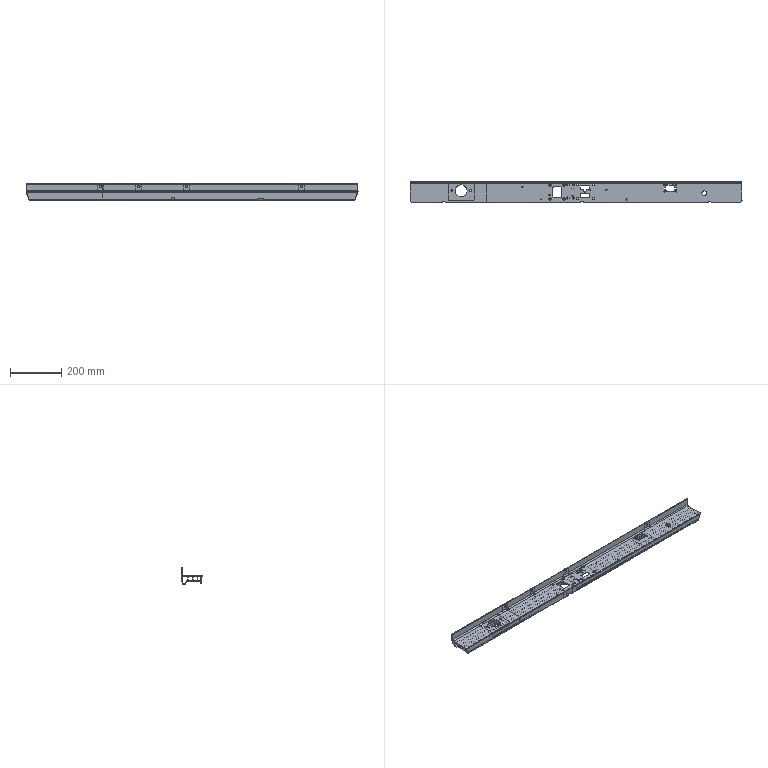NC program | NX | posted with a generic post | part box 1301 x 81.1 x 63 mm
Lines 4351 to 5403 of 19512:
(FLOOR_WALL , TOOL : D10)
N8682 T10 M6
N8684 G54
N8686 G17 G0 G90 X655.75 Y37.25 B0. C0. S6000 M3
N8688 G43 Z30. H10
N8690 Z-28.5
N8692 G94 G1 Z-30. F1000.
N8694 X653.384 Y36.253
N8696 G3 X654.25 Y35.753 R1.
N8698 G1 X450.
N8700 Y36.368
N8702 X654.25
N8704 Y36.983
N8706 X450.
N8708 Y37.597
N8710 X654.25
N8712 Y38.212
N8714 X450.
N8716 Y38.827
N8718 X654.25
N8720 Y39.442
N8722 X450.
N8724 Y40.057
N8726 X654.25
N8728 G2 X655.116 Y39.557 R1.
N8730 G1 X655.75 Y38.458
N8732 Z-28.5
N8734 G0 Z30.
N8736 X17.795 Y40.349
N8738 Z-25.5
N8740 G1 X1.001 Z-30.
N8742 X406.
N8744 Y35.75
N8746 X1.001
N8748 Z-28.5
N8750 G0 Z30.
N8752 X-169.205 Y40.349
N8754 Z-25.5
N8756 G1 X-185.999 Z-30.
N8758 X-42.999
N8760 Y35.75
N8762 X-185.999
N8764 Z-28.5
N8766 G0 Z30.
N8768 X-319.205 Y40.337
N8770 Z-25.5
N8772 G1 X-335.999 Z-30.
N8774 X-229.999
N8776 Y35.75
N8778 X-335.999
N8780 Z-28.5
N8782 G0 Z30.
N8784 X-655.748 Y41.916
N8786 Z-28.5
N8788 G1 Z-30.
N8790 X-655.114 Y40.817
N8792 G3 X-654.248 Y40.317 R1.
N8794 G1 X-379.999
N8796 Y35.75
N8798 X-654.248
N8800 G2 X-655.114 Y36.25 R1.
N8802 G1 X-655.748 Y37.348
N8804 Z-28.5
N8806 G0 Z30.
(11 , TOOL : D10)
N8808 X409.174 Y30.201 S5500
N8810 Z-9.5
N8812 G1 Z-12.5 F500.
N8814 X410.501 Y30.968
N8816 G3 X411.001 Y31.834 R1.
N8818 G1 X411. Y37.634 F1000.
N8820 Y40.25
N8822 X411.001 Y45.22
N8824 X411.002 Y45.666
N8826 G3 X410.504 Y46.534 R1.
N8828 G1 X409.176 Y47.304
N8830 Z-9.5
N8832 G0 X409.172 Y30.202 Z-22.
N8834 G1 Z-25. F500.
N8836 X410.499 Y30.968
N8838 G3 X410.999 Y31.834 R1.
N8840 G1 X411. Y37.634 F1000.
N8842 Y40.25
N8844 X410.997 Y40.577
N8846 Y44.774
N8848 X411.001 Y45.666
N8850 G3 X410.505 Y46.535 R1.
N8852 G1 X409.177 Y47.31
N8854 Z-22.
N8856 G0 Z30.
N8858 X446.825 Y47.299
N8860 Z-9.5
N8862 G1 Z-12.5 F500.
N8864 X445.498 Y46.533
N8866 G3 X444.998 Y45.666 R1.
N8868 G1 X445. Y40.25 F1000.
N8870 Y37.634
N8872 X444.998 Y31.834
N8874 G3 X445.498 Y30.968 R1.
N8876 G1 X446.826 Y30.201
N8878 Z-9.5
N8880 G0 Y47.299 Z-22.
N8882 G1 Z-25. F500.
N8884 X445.499 Y46.533
N8886 G3 X444.999 Y45.666 R1.
N8888 G1 X445. Y41.65 F1000.
N8890 X445.003 Y40.758
N8892 X444.981 Y40.687
N8894 X445.003 Y40.674
N8896 X445. Y40.25
N8898 Y37.634
N8900 X445.004 Y37.188
N8902 X445. Y31.834
N8904 G3 X445.499 Y30.967 R1.
N8906 G1 X446.827 Y30.2
N8908 Z-22.
N8910 G0 Z30.
N8912 X-39.825 Y30.201
N8914 Z-9.5
N8916 G1 Z-12.5 F500.
N8918 X-38.498 Y30.968
N8920 G3 X-37.998 Y31.834 R1.
N8922 G1 X-37.999 Y37.634 F1000.
N8924 Y40.25
N8926 X-37.998 Y45.22
N8928 X-37.997 Y45.666
N8930 G3 X-38.495 Y46.534 R1.
N8932 G1 X-39.823 Y47.304
N8934 Z-9.5
N8936 G0 X-39.827 Y30.202 Z-22.
N8938 G1 Z-25. F500.
N8940 X-38.5 Y30.968
N8942 G3 X-38. Y31.834 R1.
N8944 G1 X-37.999 Y37.634 F1000.
N8946 Y40.25
N8948 X-38.003 Y40.577
N8950 X-38.002 Y44.774
N8952 X-37.998 Y45.666
N8954 G3 X-38.494 Y46.535 R1.
N8956 G1 X-39.822 Y47.31
N8958 Z-22.
N8960 G0 Z30.
N8962 X-2.174 Y47.299
N8964 Z-9.5
N8966 G1 Z-12.5 F500.
N8968 X-3.501 Y46.533
N8970 G3 X-4.001 Y45.666 R1.
N8972 G1 X-3.999 Y40.25 F1000.
N8974 Y37.634
N8976 X-4.001 Y31.778
N8978 G3 X-3.501 Y30.912 R1.
N8980 G1 X-2.185 Y30.152
N8982 Z-9.5
N8984 G0 X-2.173 Y47.299 Z-22.
N8986 G1 Z-25. F500.
N8988 X-3.5 Y46.533
N8990 G3 X-4. Y45.666 R1.
N8992 G1 X-3.999 Y41.65 F1000.
N8994 X-3.996 Y40.758
N8996 X-4.019 Y40.687
N8998 X-3.996 Y40.674
N9000 X-3.999 Y40.25
N9002 Y37.634
N9004 X-3.996 Y37.188
N9006 X-3.999 Y31.778
N9008 G3 X-3.5 Y30.911 R1.
N9010 G1 X-2.184 Y30.151
N9012 Z-22.
N9014 G0 Z30.
N9016 X-226.825 Y30.201
N9018 Z-9.5
N9020 G1 Z-12.5 F500.
N9022 X-225.498 Y30.968
N9024 G3 X-224.998 Y31.834 R1.
N9026 G1 X-224.999 Y37.634 F1000.
N9028 Y40.25
N9030 X-224.998 Y45.22
N9032 X-224.997 Y45.666
N9034 G3 X-225.495 Y46.534 R1.
N9036 G1 X-226.823 Y47.304
N9038 Z-9.5
N9040 G0 X-226.827 Y30.2 Z-22.
N9042 G1 Z-25. F500.
N9044 X-225.499 Y30.967
N9046 G3 X-225. Y31.834 R1.
N9048 G1 X-225.003 Y37.188 F1000.
N9050 X-224.999 Y37.634
N9052 Y40.25
N9054 X-225.003 Y40.577
N9056 X-225.002 Y44.774
N9058 X-224.998 Y45.666
N9060 G3 X-225.494 Y46.535 R1.
N9062 G1 X-226.822 Y47.31
N9064 Z-22.
N9066 G0 Z30.
N9068 X-189.174 Y47.299
N9070 Z-9.5
N9072 G1 Z-12.5 F500.
N9074 X-190.501 Y46.533
N9076 G3 X-191.001 Y45.666 R1.
N9078 G1 X-190.999 Y40.25 F1000.
N9080 Y37.634
N9082 X-191.001 Y31.834
N9084 G3 X-190.501 Y30.968 R1.
N9086 G1 X-189.174 Y30.201
N9088 Z-9.5
N9090 G0 X-189.173 Y47.299 Z-22.
N9092 G1 Z-25. F500.
N9094 X-190.5 Y46.533
N9096 G3 X-191. Y45.666 R1.
N9098 G1 X-190.999 Y41.65 F1000.
N9100 X-190.996 Y40.758
N9102 X-191.019 Y40.687
N9104 X-190.996 Y40.674
N9106 X-190.999 Y40.25
N9108 Y37.634
N9110 X-190.996 Y37.188
N9112 X-190.999 Y31.834
N9114 G3 X-190.5 Y30.967 R1.
N9116 G1 X-189.172 Y30.2
N9118 Z-22.
N9120 G0 Z30.
N9122 X-376.825 Y30.201
N9124 Z-9.5
N9126 G1 Z-12.5 F500.
N9128 X-375.498 Y30.968
N9130 G3 X-374.998 Y31.834 R1.
N9132 G1 X-374.999 Y37.634 F1000.
N9134 Y40.25
N9136 X-374.998 Y45.22
N9138 X-374.997 Y45.666
N9140 G3 X-375.495 Y46.534 R1.
N9142 G1 X-376.823 Y47.304
N9144 Z-9.5
N9146 G0 X-376.827 Y30.2 Z-22.
N9148 G1 Z-25. F500.
N9150 X-375.499 Y30.967
N9152 G3 X-375. Y31.834 R1.
N9154 G1 X-375.003 Y37.188 F1000.
N9156 X-374.999 Y37.634
N9158 Y40.25
N9160 X-375.003 Y40.577
N9162 X-375.002 Y44.774
N9164 X-374.998 Y45.666
N9166 G3 X-375.494 Y46.535 R1.
N9168 G1 X-376.822 Y47.31
N9170 Z-22.
N9172 G0 Z30.
N9174 X-339.174 Y47.299
N9176 Z-9.5
N9178 G1 Z-12.5 F500.
N9180 X-340.501 Y46.533
N9182 G3 X-341.001 Y45.666 R1.
N9184 G1 X-340.999 Y40.25 F1000.
N9186 Y37.634
N9188 X-341.001 Y31.834
N9190 G3 X-340.501 Y30.968 R1.
N9192 G1 X-339.174 Y30.201
N9194 Z-9.5
N9196 G0 X-339.173 Y47.3 Z-22.
N9198 G1 Z-25. F500.
N9200 X-340.501 Y46.533
N9202 G3 X-341. Y45.666 R1.
N9204 G1 X-340.996 Y40.758 F1000.
N9206 X-341.019 Y40.687
N9208 X-340.996 Y40.674
N9210 X-340.999 Y40.25
N9212 Y37.634
N9214 X-340.996 Y37.188
N9216 X-340.999 Y31.834
N9218 G3 X-340.5 Y30.967 R1.
N9220 G1 X-339.172 Y30.2
N9222 Z-22.
N9224 G0 Z30.
(FLOOR_WALL_COPY , TOOL : D10)
N9226 X-494.633 Y32.747 S6000
N9228 Z-28.8
N9230 G1 Z-30.3
N9232 G3 X-495.5 Y33.247 R1.
N9234 G1 X-404.5
N9236 Y28.532
N9238 X-495.5
N9240 Y23.817
N9242 X-404.5
N9244 Y19.102
N9246 X-495.5
N9248 Y14.386
N9250 X-404.5
N9252 Y9.671
N9254 X-495.5
N9256 Y4.956
N9258 X-404.5
N9260 Y0.241
N9262 X-495.5
N9264 Y-4.474
N9266 X-404.5
N9268 Y-9.189
N9270 X-495.5
N9272 Y-13.905
N9274 X-404.5
N9276 Y-18.62
N9278 X-495.5
N9280 Y-23.335
N9282 X-404.5
N9284 Y-28.05
N9286 X-495.5
N9288 Y-27.184
N9290 G3 X-496. Y-28.05 R1.
N9292 G1 Y-28.55
N9294 X-404.
N9296 Y33.75
N9298 X-496.
N9300 Y-28.05
N9302 G3 X-495.75 Y-28.483 R0.5
N9304 G1 X-494.5 Y-27.05
N9306 Z-28.8
N9308 G0 Z30.
(ZLEVEL_PROFILE_COPY_2 , TOOL : D10)
N9310 X-63.3 Y5.083
N9312 Z-28.5
N9314 G1 Y15.285 Z-29.035
N9316 X-63.353 Y15.284 Z-29.038
N9318 X-85.347 Z-30.19
N9320 X-85.4 Y15.285 Z-30.193
N9322 Y-0.115 Z-31.
N9324 Y-15.516 F2000.
N9326 X-63.3
N9328 Y15.285
N9330 X-63.353 Y15.284
N9332 X-85.347
N9334 X-85.4 Y15.285
N9336 Y-0.115
N9338 Y-15.516 Z-31.269
N9340 X-63.3 Z-31.655
N9342 Y4.273 Z-32.
N9344 Y15.285
N9346 X-63.353 Y15.284
N9348 X-85.347
N9350 X-85.4 Y15.285
N9352 Y-0.115
N9354 Y-15.516 Z-32.269
N9356 X-63.3 Z-32.655
N9358 Y4.273 Z-33.
N9360 Y15.285
N9362 X-63.353 Y15.284
N9364 X-85.347
N9366 X-85.4 Y15.285
N9368 Y-15.516
N9370 X-63.3
N9372 Y4.273
N9374 Z-31.5
N9376 G0 Z30.
N9378 X47.5 Y-15.102
N9380 Z-28.5
N9382 G1 Y-10.702 Z-28.731 F1000.
N9384 X47.456 Y-10.704 Z-28.733
N9386 X22.543 Z-30.039
N9388 X22.5 Y-10.702 Z-30.041
N9390 Y-16.504 Z-30.345
N9392 X35. Z-31.
N9394 X47.5 F2000.
N9396 Y-10.702
N9398 X47.456 Y-10.704
N9400 X22.543
N9402 X22.5 Y-10.702
N9404 Y-16.504
N9406 X35.
N9408 X47.5 Z-31.271
N9410 Y-10.789 Z-31.394
N9412 Y-10.704 Z-31.396
N9414 X47.143 Z-31.404
N9416 X22.708 Z-31.933
N9418 X22.5 Z-31.937
N9420 Y-10.938 Z-31.942
N9422 Y-13.603 Z-32.
N9424 Y-16.504
N9426 X35.
N9428 X47.5 Z-32.271
N9430 Y-10.789 Z-32.394
N9432 Y-10.704 Z-32.396
N9434 X47.143 Z-32.404
N9436 X22.708 Z-32.933
N9438 X22.5 Z-32.937
N9440 Y-10.938 Z-32.942
N9442 Y-13.603 Z-33.
N9444 Y-16.504
N9446 X47.5
N9448 Y-10.702
N9450 X47.456 Y-10.704
N9452 X22.543
N9454 X22.5 Y-10.702
N9456 Y-13.603
N9458 Z-31.5
N9460 G0 Z30.
N9462 X22.827 Y14.996
N9464 Z-28.5
N9466 G1 X29.896 Z-28.871 F1000.
N9468 X30.779 Y14.87 Z-28.917
N9470 X31.631 Y14.603 Z-28.964
N9472 X32.428 Y14.203 Z-29.011
N9474 X33.15 Y13.679 Z-29.058
N9476 X33.778 Y13.046 Z-29.104
N9478 X34.296 Y12.319 Z-29.151
N9480 X34.689 Y11.519 Z-29.198
N9482 X34.949 Y10.665 Z-29.245
N9484 X35. Y10.338 Z-29.262
N9486 X35.05 Y10.665 Z-29.279
N9488 X35.31 Y11.519 Z-29.326
N9490 X35.703 Y12.319 Z-29.373
N9492 X36.221 Y13.046 Z-29.42
N9494 X36.849 Y13.679 Z-29.466
N9496 X37.571 Y14.203 Z-29.513
N9498 X38.369 Y14.603 Z-29.56
N9500 X39.22 Y14.87 Z-29.607
N9502 X40.103 Y14.996 Z-29.653
N9504 X47.5 Z-30.041
N9506 Y20.796 Z-30.345
N9508 X35. Z-31.
N9510 X22.5 F2000.
N9512 Y14.996
N9514 X29.564
N9516 G2 X35. Y10.338 R5.5
N9518 X40.435 Y14.996 R5.5
N9520 G1 X47.5
N9522 Y20.796
N9524 X35.
N9526 X22.509 Z-31.251
N9528 X22.5 Y20.582 Z-31.256
N9530 Y15.006 Z-31.368
N9532 X22.712 Y14.996 Z-31.372
N9534 X29.403 Z-31.507
N9536 X29.626 Y14.995 Z-31.511
N9538 X29.849 Y14.988 Z-31.516
N9540 X30.072 Y14.972 Z-31.52
N9542 X30.293 Y14.947 Z-31.525
N9544 X30.514 Y14.913 Z-31.529
N9546 X30.733 Y14.87 Z-31.534
N9548 X30.95 Y14.818 Z-31.538
N9550 X31.164 Y14.758 Z-31.543
N9552 X31.376 Y14.689 Z-31.547
N9554 X31.585 Y14.611 Z-31.552
N9556 X31.791 Y14.525 Z-31.556
N9558 X31.993 Y14.43 Z-31.561
N9560 X32.191 Y14.328 Z-31.565
N9562 X32.385 Y14.217 Z-31.57
N9564 X32.574 Y14.099 Z-31.574
N9566 X32.758 Y13.973 Z-31.579
N9568 X32.937 Y13.84 Z-31.583
N9570 X33.11 Y13.7 Z-31.588
N9572 X33.278 Y13.553 Z-31.592
N9574 X33.439 Y13.399 Z-31.597
N9576 X33.594 Y13.238 Z-31.601
N9578 X33.743 Y13.072 Z-31.606
N9580 X33.884 Y12.9 Z-31.61
N9582 X34.019 Y12.722 Z-31.615
N9584 X34.146 Y12.538 Z-31.619
N9586 X34.266 Y12.35 Z-31.623
N9588 X34.378 Y12.157 Z-31.628
N9590 X34.481 Y11.96 Z-31.632
N9592 X34.577 Y11.759 Z-31.637
N9594 X34.665 Y11.553 Z-31.641
N9596 X34.744 Y11.345 Z-31.646
N9598 X34.815 Y11.133 Z-31.65
N9600 X34.877 Y10.919 Z-31.655
N9602 X34.93 Y10.703 Z-31.659
N9604 X34.975 Y10.484 Z-31.664
N9606 X35.012 Y10.411 Z-31.668
N9608 X35.053 Y10.63 Z-31.673
N9610 X35.103 Y10.847 Z-31.677
N9612 X35.163 Y11.062 Z-31.682
N9614 X35.231 Y11.275 Z-31.686
N9616 X35.307 Y11.484 Z-31.691
N9618 X35.392 Y11.691 Z-31.695
N9620 X35.485 Y11.893 Z-31.7
N9622 X35.586 Y12.092 Z-31.704
N9624 X35.695 Y12.286 Z-31.709
N9626 X35.812 Y12.476 Z-31.713
N9628 X35.937 Y12.661 Z-31.718
N9630 X36.069 Y12.841 Z-31.722
N9632 X36.208 Y13.015 Z-31.727
N9634 X36.355 Y13.184 Z-31.731
N9636 X36.507 Y13.346 Z-31.736
N9638 X36.667 Y13.502 Z-31.74
N9640 X36.832 Y13.652 Z-31.745
N9642 X37.004 Y13.794 Z-31.749
N9644 X37.181 Y13.93 Z-31.754
N9646 X37.363 Y14.058 Z-31.758
N9648 X37.551 Y14.179 Z-31.762
N9650 X37.743 Y14.292 Z-31.767
N9652 X37.94 Y14.397 Z-31.771
N9654 X38.14 Y14.494 Z-31.776
N9656 X38.345 Y14.583 Z-31.78
N9658 X38.553 Y14.664 Z-31.785
N9660 X38.764 Y14.736 Z-31.789
N9662 X38.978 Y14.799 Z-31.794
N9664 X39.194 Y14.854 Z-31.798
N9666 X39.412 Y14.9 Z-31.803
N9668 X39.632 Y14.937 Z-31.807
N9670 X39.853 Y14.965 Z-31.812
N9672 X40.076 Y14.984 Z-31.816
N9674 X40.298 Y14.994 Z-31.821
N9676 X40.522 Y14.996 Z-31.825
N9678 X47.436 Z-31.964
N9680 X47.5 Y15.155 Z-31.969
N9682 Y16.716 Z-32.
N9684 Y20.796
N9686 X35.
N9688 X22.509 Z-32.251
N9690 X22.5 Y20.582 Z-32.256
N9692 Y15.006 Z-32.368
N9694 X22.712 Y14.996 Z-32.372
N9696 X29.403 Z-32.507
N9698 X29.626 Y14.995 Z-32.511
N9700 X29.849 Y14.988 Z-32.516
N9702 X30.072 Y14.972 Z-32.52
N9704 X30.293 Y14.947 Z-32.525
N9706 X30.514 Y14.913 Z-32.529
N9708 X30.733 Y14.87 Z-32.534
N9710 X30.95 Y14.818 Z-32.538
N9712 X31.164 Y14.758 Z-32.543
N9714 X31.376 Y14.689 Z-32.547
N9716 X31.585 Y14.611 Z-32.552
N9718 X31.791 Y14.525 Z-32.556
N9720 X31.993 Y14.43 Z-32.561
N9722 X32.191 Y14.328 Z-32.565
N9724 X32.385 Y14.217 Z-32.57
N9726 X32.574 Y14.099 Z-32.574
N9728 X32.758 Y13.973 Z-32.579
N9730 X32.937 Y13.84 Z-32.583
N9732 X33.11 Y13.7 Z-32.588
N9734 X33.278 Y13.553 Z-32.592
N9736 X33.439 Y13.399 Z-32.597
N9738 X33.594 Y13.238 Z-32.601
N9740 X33.743 Y13.072 Z-32.606
N9742 X33.884 Y12.9 Z-32.61
N9744 X34.019 Y12.722 Z-32.615
N9746 X34.146 Y12.538 Z-32.619
N9748 X34.266 Y12.35 Z-32.623
N9750 X34.378 Y12.157 Z-32.628
N9752 X34.481 Y11.96 Z-32.632
N9754 X34.577 Y11.759 Z-32.637
N9756 X34.665 Y11.553 Z-32.641
N9758 X34.744 Y11.345 Z-32.646
N9760 X34.815 Y11.133 Z-32.65
N9762 X34.877 Y10.919 Z-32.655
N9764 X34.93 Y10.703 Z-32.659
N9766 X34.975 Y10.484 Z-32.664
N9768 X35.012 Y10.411 Z-32.668
N9770 X35.053 Y10.63 Z-32.673
N9772 X35.103 Y10.847 Z-32.677
N9774 X35.163 Y11.062 Z-32.682
N9776 X35.231 Y11.275 Z-32.686
N9778 X35.307 Y11.484 Z-32.691
N9780 X35.392 Y11.691 Z-32.695
N9782 X35.485 Y11.893 Z-32.7
N9784 X35.586 Y12.092 Z-32.704
N9786 X35.695 Y12.286 Z-32.709
N9788 X35.812 Y12.476 Z-32.713
N9790 X35.937 Y12.661 Z-32.718
N9792 X36.069 Y12.841 Z-32.722
N9794 X36.208 Y13.015 Z-32.727
N9796 X36.355 Y13.184 Z-32.731
N9798 X36.507 Y13.346 Z-32.736
N9800 X36.667 Y13.502 Z-32.74
N9802 X36.832 Y13.652 Z-32.745
N9804 X37.004 Y13.794 Z-32.749
N9806 X37.181 Y13.93 Z-32.754
N9808 X37.363 Y14.058 Z-32.758
N9810 X37.551 Y14.179 Z-32.762
N9812 X37.743 Y14.292 Z-32.767
N9814 X37.94 Y14.397 Z-32.771
N9816 X38.14 Y14.494 Z-32.776
N9818 X38.345 Y14.583 Z-32.78
N9820 X38.553 Y14.664 Z-32.785
N9822 X38.764 Y14.736 Z-32.789
N9824 X38.978 Y14.799 Z-32.794
N9826 X39.194 Y14.854 Z-32.798
N9828 X39.412 Y14.9 Z-32.803
N9830 X39.632 Y14.937 Z-32.807
N9832 X39.853 Y14.965 Z-32.812
N9834 X40.076 Y14.984 Z-32.816
N9836 X40.298 Y14.994 Z-32.821
N9838 X40.522 Y14.996 Z-32.825
N9840 X47.436 Z-32.964
N9842 X47.5 Y15.155 Z-32.969
N9844 Y16.716 Z-33.
N9846 Y20.796
N9848 X22.5
N9850 Y14.996
N9852 X29.564
N9854 G2 X35. Y10.338 R5.5
N9856 X40.435 Y14.996 R5.5
N9858 G1 X47.5
N9860 Y16.716
N9862 Z-31.5
N9864 G0 Z30.
N9866 X363.838 Y6.914
N9868 Z-28.5
N9870 G1 X363.849 Y6.911 Z-28.501 F1000.
N9872 X364.15 Y6.785 Z-28.518
N9874 X364.292 Y6.847 Z-28.526
N9876 X364.596 Y6.964 Z-28.543
N9878 X365.224 Y7.121 Z-28.577
N9880 X365.867 Y7.2 Z-28.611
N9882 X373.419 Z-29.007
N9884 X374.141 Y7.106 Z-29.045
N9886 X374.843 Y6.913 Z-29.083
N9888 X375.143 Y6.787 Z-29.1
N9890 X375.443 Y6.913 Z-29.117
N9892 X376.146 Y7.106 Z-29.155
N9894 X376.867 Y7.2 Z-29.193
N9896 X381.835 Z-29.454
N9898 X382.144 Y7.296 Z-29.471
N9900 X382.407 Y7.486 Z-29.488
N9902 X382.597 Y7.749 Z-29.505
N9904 X382.693 Y8.058 Z-29.522
N9906 Y10.676 Z-29.659
N9908 X382.818 Y11.54 Z-29.705
N9910 X383.083 Y12.373 Z-29.75
N9912 X383.482 Y13.151 Z-29.796
N9914 X384.002 Y13.853 Z-29.842
N9916 X384.63 Y14.46 Z-29.888
N9918 X384.895 Y14.65 Z-29.905
N9920 X384.63 Y14.84 Z-29.922
N9922 X384.002 Y15.447 Z-29.968
N9924 X383.482 Y16.149 Z-30.014
N9926 X383.083 Y16.927 Z-30.059
N9928 X382.818 Y17.76 Z-30.105
N9930 X382.693 Y18.624 Z-30.151
N9932 Y21.242 Z-30.288
N9934 X382.59 Y21.563 Z-30.306
N9936 X382.388 Y21.833 Z-30.324
N9938 X382.107 Y22.021 Z-30.341
N9940 X381.667 Y22.149 Z-30.365
N9942 X381.387 Y22.259 Z-30.381
N9944 X381.105 Y22.401 Z-30.398
N9946 X380.797 Y22.293 Z-30.415
N9948 X380.238 Y22.166 Z-30.445
N9950 X379.669 Y22.1 Z-30.475
N9952 X369.643 Z-31.
N9954 X359.943 F2000.
N9956 G2 X358.188 Y22.399 R5.3
N9958 X357.315 Y22.061 R5.3
N9960 G3 X356.593 Y21.1 R1.
N9962 G1 Y18.95
N9964 G2 X354.391 Y14.65 R5.3
N9966 X356.593 Y10.35 R5.3
N9968 G1 Y8.2
N9970 G3 X357.593 Y7.2 R1.
N9972 G1 X362.093
N9974 G2 X364.15 Y6.785 R5.3
N9976 G1 X364.292 Y6.847
N9978 G2 X366.193 Y7.2 R5.3
N9980 G1 X373.093
N9982 G2 X375.143 Y6.787 R5.3
N9984 X377.193 Y7.2 R5.3
N9986 G1 X381.693
N9988 G3 X382.693 Y8.2 R1.
N9990 G1 Y10.35
N9992 G2 X384.895 Y14.65 R5.3
N9994 X382.693 Y18.95 R5.3
N9996 G1 Y21.1
N9998 G3 X381.971 Y22.061 R1.
N10000 G2 X381.105 Y22.401 R5.
N10002 X379.343 Y22.1 R5.3
N10004 G1 X369.643
N10006 X360.095 Z-31.167
N10008 X359.873 Z-31.171
N10010 X359.651 Y22.108 Z-31.175
N10012 X359.429 Y22.125 Z-31.178
N10014 X359.209 Y22.151 Z-31.182
N10016 X358.99 Y22.186 Z-31.186
N10018 X358.772 Y22.232 Z-31.19
N10020 X358.557 Y22.285 Z-31.194
N10022 X358.451 Y22.314 Z-31.196
N10024 X358.345 Y22.347 Z-31.198
N10026 X358.291 Y22.364 Z-31.199
N10028 X358.212 Y22.391 Z-31.2
N10030 X358.185 Y22.398 Z-31.201
N10032 X358.136 Y22.374 Z-31.202
N10034 X357.934 Y22.282 Z-31.206
N10036 X357.728 Y22.199 Z-31.209
N10038 X357.519 Y22.124 Z-31.213
N10040 X357.309 Y22.052 Z-31.217
N10042 X357.115 Y21.97 Z-31.221
N10044 X357.027 Y21.917 Z-31.223
N10046 X356.927 Y21.837 Z-31.225
N10048 X356.805 Y21.706 Z-31.228
N10050 X356.756 Y21.633 Z-31.23
N10052 X356.726 Y21.584 Z-31.231
N10054 X356.675 Y21.48 Z-31.233
N10056 X356.631 Y21.372 Z-31.235
N10058 X356.617 Y21.316 Z-31.236
N10060 X356.608 Y21.227 Z-31.237
N10062 X356.596 Y21.048 Z-31.24
N10064 X356.593 Y20.826 Z-31.244
N10066 Y19.272 Z-31.271
N10068 Y19.05 Z-31.275
N10070 X356.592 Y18.828 Z-31.279
N10072 X356.582 Y18.606 Z-31.283
N10074 X356.563 Y18.384 Z-31.287
N10076 X356.534 Y18.164 Z-31.291
N10078 X356.497 Y17.945 Z-31.295
N10080 X356.449 Y17.729 Z-31.299
N10082 X356.395 Y17.513 Z-31.302
N10084 X356.33 Y17.301 Z-31.306
N10086 X356.256 Y17.091 Z-31.31
N10088 X356.174 Y16.885 Z-31.314
N10090 X356.084 Y16.683 Z-31.318
N10092 X355.984 Y16.484 Z-31.322
N10094 X355.877 Y16.29 Z-31.326
N10096 X355.761 Y16.1 Z-31.33
N10098 X355.638 Y15.915 Z-31.333
N10100 X355.507 Y15.736 Z-31.337
N10102 X355.369 Y15.562 Z-31.341
N10104 X355.223 Y15.394 Z-31.345
N10106 X355.071 Y15.233 Z-31.349
N10108 X354.912 Y15.078 Z-31.353
N10110 X354.747 Y14.93 Z-31.357
N10112 X354.398 Y14.655 Z-31.365
N10114 X354.734 Y14.381 Z-31.372
N10116 X354.9 Y14.233 Z-31.376
N10118 X355.059 Y14.079 Z-31.38
N10120 X355.212 Y13.918 Z-31.384
N10122 X355.358 Y13.75 Z-31.388
N10124 X355.497 Y13.577 Z-31.392
N10126 X355.629 Y13.398 Z-31.396
N10128 X355.753 Y13.214 Z-31.399
N10130 X355.869 Y13.025 Z-31.403
N10132 X355.977 Y12.831 Z-31.407
N10134 X356.076 Y12.632 Z-31.411
N10136 X356.168 Y12.43 Z-31.415
N10138 X356.251 Y12.224 Z-31.419
N10140 X356.325 Y12.015 Z-31.423
N10142 X356.39 Y11.803 Z-31.427
N10144 X356.446 Y11.588 Z-31.43
N10146 X356.494 Y11.371 Z-31.434
N10148 X356.532 Y11.152 Z-31.438
N10150 X356.561 Y10.932 Z-31.442
N10152 X356.581 Y10.711 Z-31.446
N10154 X356.591 Y10.489 Z-31.45
N10156 X356.593 Y10.267 Z-31.454
N10158 Y10.045 Z-31.458
N10160 Y8.491 Z-31.485
N10162 X356.596 Y8.268 Z-31.489
N10164 X356.613 Y8.053 Z-31.492
N10166 X356.634 Y7.949 Z-31.494
N10168 X356.644 Y7.911 Z-31.495
N10170 X356.671 Y7.836 Z-31.496
N10172 X356.754 Y7.668 Z-31.5
N10174 X356.807 Y7.592 Z-31.501
N10176 X356.841 Y7.552 Z-31.502
N10178 X356.916 Y7.475 Z-31.504
N10180 X357.056 Y7.365 Z-31.507
N10182 X357.132 Y7.321 Z-31.509
N10184 X357.184 Y7.297 Z-31.51
N10186 X357.293 Y7.255 Z-31.512
N10188 X357.391 Y7.229 Z-31.514
N10190 X357.441 Y7.221
N10192 X357.537 Y7.211 Z-31.516
N10194 X357.73 Y7.2 Z-31.52
N10196 X361.949 Z-31.593
N10198 X362.171 Y7.199 Z-31.597
N10200 X362.393 Y7.191 Z-31.601
N10202 X362.615 Y7.174 Z-31.605
N10204 X362.835 Y7.148 Z-31.609
N10206 X363.054 Y7.112 Z-31.613
N10208 X363.272 Y7.067 Z-31.616
N10210 X363.487 Y7.013 Z-31.62
N10212 X363.7 Y6.951 Z-31.624
N10214 X363.91 Y6.879 Z-31.628
N10216 X364.142 Y6.788 Z-31.632
N10218 X364.321 Y6.858 Z-31.636
N10220 X364.531 Y6.932 Z-31.64
N10222 X364.743 Y6.998 Z-31.644
N10224 X364.958 Y7.053 Z-31.647
N10226 X365.175 Y7.101 Z-31.651
N10228 X365.393 Y7.139 Z-31.655
N10230 X365.613 Y7.168 Z-31.659
N10232 X365.835 Y7.188 Z-31.663
N10234 X366.056 Y7.198 Z-31.667
N10236 X366.278 Y7.2 Z-31.671
N10238 X366.5 Z-31.675
N10240 X372.94 Z-31.787
N10242 X373.162 Z-31.791
N10244 X373.384 Y7.192 Z-31.795
N10246 X373.605 Y7.175 Z-31.799
N10248 X373.826 Y7.149 Z-31.802
N10250 X374.045 Y7.114 Z-31.806
N10252 X374.263 Y7.069 Z-31.81
N10254 X374.478 Y7.016 Z-31.814
N10256 X374.691 Y6.953 Z-31.818
N10258 X374.901 Y6.882 Z-31.822
N10260 X375.144 Y6.787 Z-31.826
N10262 X375.315 Y6.856 Z-31.83
N10264 X375.524 Y6.93 Z-31.833
N10266 X375.736 Y6.996 Z-31.837
N10268 X375.951 Y7.051 Z-31.841
N10270 X376.168 Y7.1 Z-31.845
N10272 X376.386 Y7.137 Z-31.849
N10274 X376.606 Y7.167 Z-31.853
N10276 X376.827 Y7.187 Z-31.857
N10278 X377.049 Y7.198 Z-31.861
N10280 X377.271 Y7.2 Z-31.865
N10282 X377.493 Z-31.868
N10284 X381.49 Z-31.938
N10286 X381.734 Y7.209 Z-31.942
N10288 X381.854 Y7.221 Z-31.945
N10290 X381.93 Y7.236 Z-31.946
N10292 X382.103 Y7.296 Z-31.949
N10294 X382.182 Y7.338 Z-31.951
N10296 X382.23 Y7.366 Z-31.952
N10298 X382.322 Y7.431 Z-31.954
N10300 X382.449 Y7.557 Z-31.957
N10302 X382.535 Y7.674 Z-31.959
N10304 X382.591 Y7.776 Z-31.961
N10306 X382.636 Y7.891 Z-31.964
N10308 X382.653 Y7.951 Z-31.965
N10310 X382.671 Y8.033 Z-31.966
N10312 X382.686 Y8.203 Z-31.969
N10314 X382.693 Y8.425 Z-31.973
N10316 Y9.979 Z-32.
N10318 Y10.35
N10320 G2 X384.895 Y14.65 R5.3
N10322 X382.693 Y18.95 R5.3
N10324 G1 Y21.1
N10326 G3 X381.971 Y22.061 R1.
N10328 G2 X381.105 Y22.401 R5.
N10330 X379.343 Y22.1 R5.3
N10332 G1 X369.643
N10334 X360.095 Z-32.167
N10336 X359.873 Z-32.171
N10338 X359.651 Y22.108 Z-32.175
N10340 X359.429 Y22.125 Z-32.178
N10342 X359.209 Y22.151 Z-32.182
N10344 X358.99 Y22.186 Z-32.186
N10346 X358.772 Y22.232 Z-32.19
N10348 X358.557 Y22.285 Z-32.194
N10350 X358.451 Y22.314 Z-32.196
N10352 X358.345 Y22.347 Z-32.198
N10354 X358.291 Y22.364 Z-32.199
N10356 X358.212 Y22.391 Z-32.2
N10358 X358.185 Y22.398 Z-32.201
N10360 X358.136 Y22.374 Z-32.202
N10362 X357.934 Y22.282 Z-32.206
N10364 X357.728 Y22.199 Z-32.209
N10366 X357.519 Y22.124 Z-32.213
N10368 X357.309 Y22.052 Z-32.217
N10370 X357.115 Y21.97 Z-32.221
N10372 X357.027 Y21.917 Z-32.223
N10374 X356.927 Y21.837 Z-32.225
N10376 X356.805 Y21.706 Z-32.228
N10378 X356.756 Y21.633 Z-32.23
N10380 X356.726 Y21.584 Z-32.231
N10382 X356.675 Y21.48 Z-32.233
N10384 X356.638 Y21.37 Z-32.235
N10386 X356.622 Y21.315 Z-32.236
N10388 X356.608 Y21.227 Z-32.237
N10390 X356.596 Y21.048 Z-32.24
N10392 X356.593 Y20.826 Z-32.244
N10394 Y19.272 Z-32.271
N10396 Y19.05 Z-32.275
N10398 X356.592 Y18.828 Z-32.279
N10400 X356.582 Y18.606 Z-32.283
N10402 X356.563 Y18.384 Z-32.287
N10404 X356.534 Y18.164 Z-32.291
N10406 X356.497 Y17.945 Z-32.295
N10408 X356.45 Y17.728 Z-32.299
N10410 X356.395 Y17.513 Z-32.302
N10412 X356.33 Y17.301 Z-32.306
N10414 X356.256 Y17.091 Z-32.31
N10416 X356.174 Y16.885 Z-32.314
N10418 X356.084 Y16.683 Z-32.318
N10420 X355.984 Y16.484 Z-32.322
N10422 X355.877 Y16.29 Z-32.326
N10424 X355.761 Y16.1 Z-32.33
N10426 X355.638 Y15.915 Z-32.333
N10428 X355.507 Y15.736 Z-32.337
N10430 X355.369 Y15.562 Z-32.341
N10432 X355.223 Y15.394 Z-32.345
N10434 X355.071 Y15.233 Z-32.349
N10436 X354.912 Y15.078 Z-32.353
N10438 X354.747 Y14.93 Z-32.357
N10440 X354.398 Y14.655 Z-32.365
N10442 X354.734 Y14.381 Z-32.372
N10444 X354.9 Y14.233 Z-32.376
N10446 X355.059 Y14.079 Z-32.38
N10448 X355.212 Y13.918 Z-32.384
N10450 X355.358 Y13.75 Z-32.388
N10452 X355.497 Y13.577 Z-32.392
N10454 X355.629 Y13.398 Z-32.396
N10456 X355.753 Y13.214 Z-32.399
N10458 X355.869 Y13.025 Z-32.403
N10460 X355.977 Y12.831 Z-32.407
N10462 X356.076 Y12.632 Z-32.411
N10464 X356.168 Y12.43 Z-32.415
N10466 X356.251 Y12.224 Z-32.419
N10468 X356.325 Y12.015 Z-32.423
N10470 X356.39 Y11.803 Z-32.427
N10472 X356.446 Y11.588 Z-32.43
N10474 X356.494 Y11.371 Z-32.434
N10476 X356.532 Y11.152 Z-32.438
N10478 X356.561 Y10.932 Z-32.442
N10480 X356.581 Y10.711 Z-32.446
N10482 X356.591 Y10.489 Z-32.45
N10484 X356.593 Y10.267 Z-32.454
N10486 Y10.045 Z-32.458
N10488 Y8.491 Z-32.485
N10490 X356.596 Y8.268 Z-32.489
N10492 X356.613 Y8.053 Z-32.492
N10494 X356.634 Y7.949 Z-32.494
N10496 X356.644 Y7.91 Z-32.495
N10498 X356.671 Y7.836 Z-32.496
N10500 X356.754 Y7.668 Z-32.5
N10502 X356.807 Y7.593 Z-32.501
N10504 X356.841 Y7.552 Z-32.502
N10506 X356.916 Y7.475 Z-32.504
N10508 X357.056 Y7.365 Z-32.507
N10510 X357.132 Y7.321 Z-32.509
N10512 X357.184 Y7.297 Z-32.51
N10514 X357.293 Y7.255 Z-32.512
N10516 X357.391 Y7.229 Z-32.514
N10518 X357.441 Y7.221
N10520 X357.537 Y7.211 Z-32.516
N10522 X357.73 Y7.2 Z-32.52
N10524 X361.949 Z-32.593
N10526 X362.171 Y7.199 Z-32.597
N10528 X362.393 Y7.191 Z-32.601
N10530 X362.615 Y7.174 Z-32.605
N10532 X362.835 Y7.148 Z-32.609
N10534 X363.054 Y7.112 Z-32.613
N10536 X363.272 Y7.067 Z-32.616
N10538 X363.487 Y7.013 Z-32.62
N10540 X363.7 Y6.951 Z-32.624
N10542 X363.91 Y6.879 Z-32.628
N10544 X364.142 Y6.788 Z-32.632
N10546 X364.321 Y6.858 Z-32.636
N10548 X364.531 Y6.932 Z-32.64
N10550 X364.743 Y6.998 Z-32.644
N10552 X364.958 Y7.054 Z-32.647
N10554 X365.175 Y7.101 Z-32.651
N10556 X365.393 Y7.139 Z-32.655
N10558 X365.613 Y7.168 Z-32.659
N10560 X365.835 Y7.188 Z-32.663
N10562 X366.056 Y7.198 Z-32.667
N10564 X366.278 Y7.2 Z-32.671
N10566 X366.5 Z-32.675
N10568 X372.94 Z-32.787
N10570 X373.162 Z-32.791
N10572 X373.384 Y7.192 Z-32.795
N10574 X373.605 Y7.175 Z-32.799
N10576 X373.826 Y7.149 Z-32.802
N10578 X374.045 Y7.114 Z-32.806
N10580 X374.263 Y7.069 Z-32.81
N10582 X374.478 Y7.016 Z-32.814
N10584 X374.691 Y6.953 Z-32.818
N10586 X374.901 Y6.882 Z-32.822
N10588 X375.144 Y6.787 Z-32.826
N10590 X375.315 Y6.856 Z-32.83
N10592 X375.524 Y6.93 Z-32.833
N10594 X375.736 Y6.996 Z-32.837
N10596 X375.951 Y7.051 Z-32.841
N10598 X376.168 Y7.1 Z-32.845
N10600 X376.386 Y7.138 Z-32.849
N10602 X376.606 Y7.167 Z-32.853
N10604 X376.827 Y7.187 Z-32.857
N10606 X377.049 Y7.198 Z-32.861
N10608 X377.271 Y7.2 Z-32.865
N10610 X377.493 Z-32.868
N10612 X381.49 Z-32.938
N10614 X381.734 Y7.209 Z-32.942
N10616 X381.854 Y7.221 Z-32.945
N10618 X381.93 Y7.236 Z-32.946
N10620 X382.103 Y7.296 Z-32.949
N10622 X382.182 Y7.338 Z-32.951
N10624 X382.23 Y7.366 Z-32.952
N10626 X382.322 Y7.431 Z-32.954
N10628 X382.449 Y7.557 Z-32.957
N10630 X382.535 Y7.674 Z-32.959
N10632 X382.591 Y7.776 Z-32.961
N10634 X382.636 Y7.891 Z-32.964
N10636 X382.653 Y7.951 Z-32.965
N10638 X382.671 Y8.033 Z-32.966
N10640 X382.686 Y8.203 Z-32.969
N10642 X382.693 Y8.425 Z-32.973
N10644 Y9.979 Z-33.
N10646 Y10.35
N10648 G2 X384.895 Y14.65 R5.3
N10650 X382.693 Y18.95 R5.3
N10652 G1 Y21.1
N10654 G3 X381.971 Y22.061 R1.
N10656 G2 X381.105 Y22.401 R5.
N10658 X379.343 Y22.1 R5.3
N10660 G1 X359.943
N10662 G2 X358.188 Y22.399 R5.3
N10664 X357.315 Y22.061 R5.3
N10666 G3 X356.593 Y21.1 R1.
N10668 G1 Y18.95
N10670 G2 X354.391 Y14.65 R5.3
N10672 X356.593 Y10.35 R5.3
N10674 G1 Y8.2
N10676 G3 X357.593 Y7.2 R1.
N10678 G1 X362.093
N10680 G2 X364.145 Y6.787 R5.3
N10682 G1 X364.281 Y6.842
N10684 X364.292 Y6.847
N10686 G2 X366.193 Y7.2 R5.3
N10688 G1 X373.093
N10690 G2 X375.143 Y6.787 R5.3
N10692 X377.193 Y7.2 R5.3
N10694 G1 X381.693
N10696 G3 X382.693 Y8.2 R1.
N10698 G1 Y9.979
N10700 Z-31.5
N10702 G0 Z30.
(HOLE_MILLING_1_COPY_1 , TOOL : D10)
N10704 X-518.498 Y-43.55
N10706 Z-29.5
N10708 G3 X-517.498 Y-44.55 R1. F1400.
N10710 X-516.498 Y-43.55 R1.
N10712 X-516.498 Y-43.55 Z-30.5 I-2. J0.
N10714 X-516.498 Y-43.55 Z-31.5 I-2. J0.
N10716 X-516.498 Y-43.55 Z-32.5 I-2. J0.
N10718 X-520.498 Y-43.55 Z-33. I-2. J0.
N10720 X-518.498 Y-45.55 R2.
N10722 X-520.498 Y-43.55 R-2.
N10724 X-519.498 Y-44.55 R1.
N10726 X-518.498 Y-43.55 R1.
N10728 G0 Z30.
N10730 X23.5
N10732 Z-29.5
N10734 G3 X24.5 Y-44.55 R1.
N10736 X25.5 Y-43.55 R1.
N10738 X25.5 Y-43.55 Z-30.5 I-2. J0.
N10740 X25.5 Y-43.55 Z-31.5 I-2. J0.
N10742 X25.5 Y-43.55 Z-32.5 I-2. J0.
N10744 X21.5 Y-43.55 Z-33. I-2. J0.
N10746 X23.5 Y-45.55 R2.
N10748 X21.5 Y-43.55 R-2.
N10750 X22.5 Y-44.55 R1.
N10752 X23.5 Y-43.55 R1.
N10754 G0 Z30.
N10756 M5